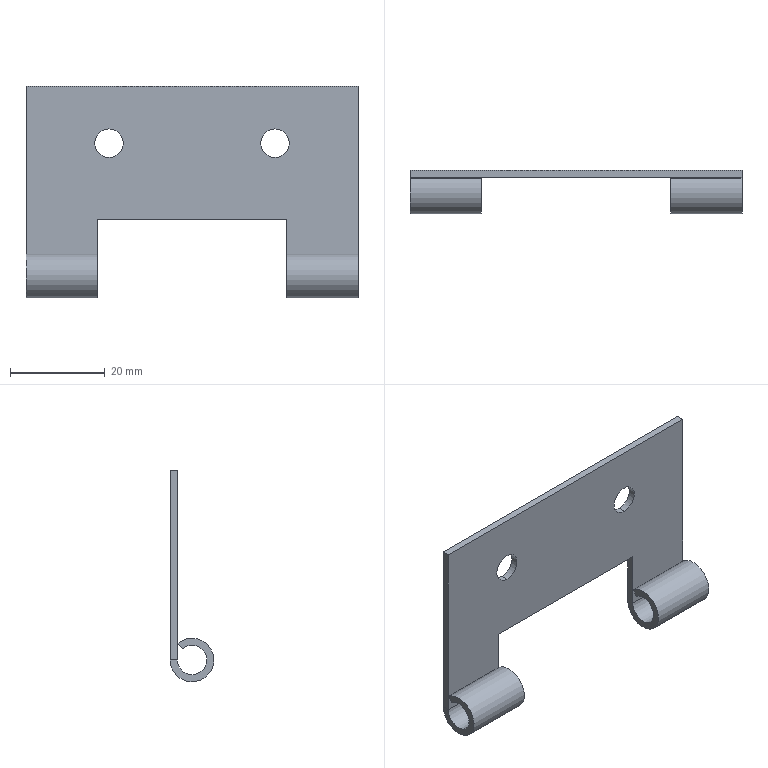Part | NX | features BREP 1 | 1 solid | 20 faces | box 70 x 9.2 x 44.6 mm | volume 4333 mm3 | plane 12 | cylinder 8 | commonest cylinder face diameters 6 x4 6.2 x2 9.2 x2
STEP:
#1=CARTESIAN_POINT('',(-20.,-1.5,-8.));
#2=VERTEX_POINT('',#1);
#3=CARTESIAN_POINT('',(-20.,-1.5,-20.));
#4=VERTEX_POINT('',#3);
#5=CARTESIAN_POINT('',(-20.,-1.5,-8.));
#6=DIRECTION('',(0.,0.,-1.));
#7=VECTOR('',#6,1000.);
#8=LINE('',#5,#7);
#9=EDGE_CURVE('',#2,#4,#8,.T.);
#10=ORIENTED_EDGE('',*,*,#9,.F.);
#11=CARTESIAN_POINT('',(20.,-1.5,-8.));
#12=VERTEX_POINT('',#11);
#13=CARTESIAN_POINT('',(20.,-1.5,-8.));
#14=DIRECTION('',(-1.,0.,0.));
#15=VECTOR('',#14,1000.);
#16=LINE('',#13,#15);
#17=EDGE_CURVE('',#12,#2,#16,.T.);
#18=ORIENTED_EDGE('',*,*,#17,.F.);
#19=CARTESIAN_POINT('',(20.,-1.5,-20.));
#20=VERTEX_POINT('',#19);
#21=CARTESIAN_POINT('',(20.,-1.5,-20.));
#22=DIRECTION('',(0.,0.,1.));
#23=VECTOR('',#22,1000.);
#24=LINE('',#21,#23);
#25=EDGE_CURVE('',#20,#12,#24,.T.);
#26=ORIENTED_EDGE('',*,*,#25,.F.);
#27=CARTESIAN_POINT('',(35.,-1.5,-20.));
#28=VERTEX_POINT('',#27);
#29=CARTESIAN_POINT('',(20.,-1.5,-20.));
#30=DIRECTION('',(1.,0.,0.));
#31=VECTOR('',#30,1000.);
#32=LINE('',#29,#31);
#33=EDGE_CURVE('',#20,#28,#32,.T.);
#34=ORIENTED_EDGE('',*,*,#33,.T.);
#35=CARTESIAN_POINT('',(35.,-1.5,20.));
#36=VERTEX_POINT('',#35);
#37=CARTESIAN_POINT('',(35.,-1.5,20.));
#38=DIRECTION('',(0.,0.,-1.));
#39=VECTOR('',#38,1000.);
#40=LINE('',#37,#39);
#41=EDGE_CURVE('',#36,#28,#40,.T.);
#42=ORIENTED_EDGE('',*,*,#41,.F.);
#43=CARTESIAN_POINT('',(-35.,-1.5,20.));
#44=VERTEX_POINT('',#43);
#45=CARTESIAN_POINT('',(-35.,-1.5,20.));
#46=DIRECTION('',(1.,0.,0.));
#47=VECTOR('',#46,1000.);
#48=LINE('',#45,#47);
#49=EDGE_CURVE('',#44,#36,#48,.T.);
#50=ORIENTED_EDGE('',*,*,#49,.F.);
#51=CARTESIAN_POINT('',(-35.,-1.5,-20.));
#52=VERTEX_POINT('',#51);
#53=CARTESIAN_POINT('',(-35.,-1.5,-20.));
#54=DIRECTION('',(0.,0.,1.));
#55=VECTOR('',#54,1000.);
#56=LINE('',#53,#55);
#57=EDGE_CURVE('',#52,#44,#56,.T.);
#58=ORIENTED_EDGE('',*,*,#57,.F.);
#59=CARTESIAN_POINT('',(-35.,-1.5,-20.));
#60=DIRECTION('',(1.,0.,0.));
#61=VECTOR('',#60,1000.);
#62=LINE('',#59,#61);
#63=EDGE_CURVE('',#52,#4,#62,.T.);
#64=ORIENTED_EDGE('',*,*,#63,.T.);
#65=EDGE_LOOP('',(#10,#18,#26,#34,#42,#50,#58,#64));
#66=FACE_BOUND('',#65,.T.);
#67=CARTESIAN_POINT('',(17.5,-1.5,5.));
#68=VERTEX_POINT('',#67);
#69=CARTESIAN_POINT('',(17.5,-1.5,11.));
#70=VERTEX_POINT('',#69);
#71=CARTESIAN_POINT('',(17.5,-1.5,8.));
#72=DIRECTION('',(0.,-1.,0.));
#73=DIRECTION('',(0.,0.,-1.));
#74=AXIS2_PLACEMENT_3D('',#71,#72,#73);
#75=CIRCLE('',#74,3.);
#76=EDGE_CURVE('',#68,#70,#75,.T.);
#77=ORIENTED_EDGE('',*,*,#76,.F.);
#78=CARTESIAN_POINT('',(17.5,-1.5,8.));
#79=DIRECTION('',(0.,-1.,0.));
#80=DIRECTION('',(0.,0.,1.));
#81=AXIS2_PLACEMENT_3D('',#78,#79,#80);
#82=CIRCLE('',#81,3.);
#83=EDGE_CURVE('',#70,#68,#82,.T.);
#84=ORIENTED_EDGE('',*,*,#83,.F.);
#85=EDGE_LOOP('',(#77,#84));
#86=FACE_BOUND('',#85,.T.);
#87=CARTESIAN_POINT('',(-17.5,-1.5,5.));
#88=VERTEX_POINT('',#87);
#89=CARTESIAN_POINT('',(-17.5,-1.5,11.));
#90=VERTEX_POINT('',#89);
#91=CARTESIAN_POINT('',(-17.5,-1.5,8.));
#92=DIRECTION('',(0.,-1.,0.));
#93=DIRECTION('',(0.,0.,-1.));
#94=AXIS2_PLACEMENT_3D('',#91,#92,#93);
#95=CIRCLE('',#94,3.);
#96=EDGE_CURVE('',#88,#90,#95,.T.);
#97=ORIENTED_EDGE('',*,*,#96,.F.);
#98=CARTESIAN_POINT('',(-17.5,-1.5,8.));
#99=DIRECTION('',(0.,-1.,0.));
#100=DIRECTION('',(0.,0.,1.));
#101=AXIS2_PLACEMENT_3D('',#98,#99,#100);
#102=CIRCLE('',#101,3.);
#103=EDGE_CURVE('',#90,#88,#102,.T.);
#104=ORIENTED_EDGE('',*,*,#103,.F.);
#105=EDGE_LOOP('',(#97,#104));
#106=FACE_BOUND('',#105,.T.);
#107=CARTESIAN_POINT('',(0.,-1.5,0.));
#108=DIRECTION('',(0.,-1.,0.));
#109=DIRECTION('',(0.,0.,-1.));
#110=AXIS2_PLACEMENT_3D('',#107,#108,#109);
#111=PLANE('',#110);
#112=ADVANCED_FACE('',(#66,#86,#106),#111,.T.);
#113=CARTESIAN_POINT('',(-20.,-2.607,-17.625));
#114=VERTEX_POINT('',#113);
#115=CARTESIAN_POINT('',(-20.,-4.6,-20.));
#116=DIRECTION('',(1.,0.,0.));
#117=DIRECTION('',(0.,0.,1.));
#118=AXIS2_PLACEMENT_3D('',#115,#116,#117);
#119=CIRCLE('',#118,3.1);
#120=EDGE_CURVE('',#114,#4,#119,.T.);
#121=ORIENTED_EDGE('',*,*,#120,.T.);
#122=ORIENTED_EDGE('',*,*,#63,.F.);
#123=CARTESIAN_POINT('',(-35.,-2.607,-17.625));
#124=VERTEX_POINT('',#123);
#125=CARTESIAN_POINT('',(-35.,-4.6,-20.));
#126=DIRECTION('',(-1.,0.,0.));
#127=DIRECTION('',(0.,1.,0.));
#128=AXIS2_PLACEMENT_3D('',#125,#126,#127);
#129=CIRCLE('',#128,3.1);
#130=EDGE_CURVE('',#52,#124,#129,.T.);
#131=ORIENTED_EDGE('',*,*,#130,.T.);
#132=CARTESIAN_POINT('',(-20.,-2.607,-17.625));
#133=DIRECTION('',(-1.,0.,0.));
#134=VECTOR('',#133,1000.);
#135=LINE('',#132,#134);
#136=EDGE_CURVE('',#114,#124,#135,.T.);
#137=ORIENTED_EDGE('',*,*,#136,.F.);
#138=EDGE_LOOP('',(#121,#122,#131,#137));
#139=FACE_BOUND('',#138,.T.);
#140=CARTESIAN_POINT('',(35.,-4.6,-20.));
#141=DIRECTION('',(1.,0.,0.));
#142=DIRECTION('',(0.,0.6428,0.766));
#143=AXIS2_PLACEMENT_3D('',#140,#141,#142);
#144=CYLINDRICAL_SURFACE('',#143,3.1);
#145=ADVANCED_FACE('',(#139),#144,.F.);
#146=CARTESIAN_POINT('',(-20.,0.,-8.));
#147=VERTEX_POINT('',#146);
#148=CARTESIAN_POINT('',(-20.,-1.5,-8.));
#149=DIRECTION('',(0.,1.,0.));
#150=VECTOR('',#149,1000.);
#151=LINE('',#148,#150);
#152=EDGE_CURVE('',#2,#147,#151,.T.);
#153=ORIENTED_EDGE('',*,*,#152,.F.);
#154=ORIENTED_EDGE('',*,*,#9,.T.);
#155=ORIENTED_EDGE('',*,*,#120,.F.);
#156=CARTESIAN_POINT('',(-20.,-1.643,-16.476));
#157=VERTEX_POINT('',#156);
#158=CARTESIAN_POINT('',(-20.,-1.643,-16.476));
#159=DIRECTION('',(0.,-0.6428,-0.766));
#160=VECTOR('',#159,1000.);
#161=LINE('',#158,#160);
#162=EDGE_CURVE('',#157,#114,#161,.T.);
#163=ORIENTED_EDGE('',*,*,#162,.F.);
#164=CARTESIAN_POINT('',(-20.,0.,-20.));
#165=VERTEX_POINT('',#164);
#166=CARTESIAN_POINT('',(-20.,-4.6,-20.));
#167=DIRECTION('',(-1.,0.,0.));
#168=DIRECTION('',(0.,0.,1.));
#169=AXIS2_PLACEMENT_3D('',#166,#167,#168);
#170=CIRCLE('',#169,4.6);
#171=EDGE_CURVE('',#165,#157,#170,.T.);
#172=ORIENTED_EDGE('',*,*,#171,.F.);
#173=CARTESIAN_POINT('',(-20.,0.,-20.));
#174=DIRECTION('',(0.,0.,1.));
#175=VECTOR('',#174,1000.);
#176=LINE('',#173,#175);
#177=EDGE_CURVE('',#165,#147,#176,.T.);
#178=ORIENTED_EDGE('',*,*,#177,.T.);
#179=EDGE_LOOP('',(#153,#154,#155,#163,#172,#178));
#180=FACE_BOUND('',#179,.T.);
#181=CARTESIAN_POINT('',(-20.,0.,-59.596));
#182=DIRECTION('',(1.,0.,0.));
#183=DIRECTION('',(0.,1.,0.));
#184=AXIS2_PLACEMENT_3D('',#181,#182,#183);
#185=PLANE('',#184);
#186=ADVANCED_FACE('',(#180),#185,.T.);
#187=CARTESIAN_POINT('',(-35.,0.,-20.));
#188=VERTEX_POINT('',#187);
#189=CARTESIAN_POINT('',(-20.,0.,-20.));
#190=DIRECTION('',(-1.,0.,0.));
#191=VECTOR('',#190,1000.);
#192=LINE('',#189,#191);
#193=EDGE_CURVE('',#165,#188,#192,.T.);
#194=ORIENTED_EDGE('',*,*,#193,.T.);
#195=CARTESIAN_POINT('',(-35.,0.,20.));
#196=VERTEX_POINT('',#195);
#197=CARTESIAN_POINT('',(-35.,0.,20.));
#198=DIRECTION('',(0.,0.,-1.));
#199=VECTOR('',#198,1000.);
#200=LINE('',#197,#199);
#201=EDGE_CURVE('',#196,#188,#200,.T.);
#202=ORIENTED_EDGE('',*,*,#201,.F.);
#203=CARTESIAN_POINT('',(35.,0.,20.));
#204=VERTEX_POINT('',#203);
#205=CARTESIAN_POINT('',(35.,0.,20.));
#206=DIRECTION('',(-1.,0.,0.));
#207=VECTOR('',#206,1000.);
#208=LINE('',#205,#207);
#209=EDGE_CURVE('',#204,#196,#208,.T.);
#210=ORIENTED_EDGE('',*,*,#209,.F.);
#211=CARTESIAN_POINT('',(35.,0.,-20.));
#212=VERTEX_POINT('',#211);
#213=CARTESIAN_POINT('',(35.,0.,-20.));
#214=DIRECTION('',(0.,0.,1.));
#215=VECTOR('',#214,1000.);
#216=LINE('',#213,#215);
#217=EDGE_CURVE('',#212,#204,#216,.T.);
#218=ORIENTED_EDGE('',*,*,#217,.F.);
#219=CARTESIAN_POINT('',(20.,0.,-20.));
#220=VERTEX_POINT('',#219);
#221=CARTESIAN_POINT('',(35.,0.,-20.));
#222=DIRECTION('',(-1.,0.,0.));
#223=VECTOR('',#222,1000.);
#224=LINE('',#221,#223);
#225=EDGE_CURVE('',#212,#220,#224,.T.);
#226=ORIENTED_EDGE('',*,*,#225,.T.);
#227=CARTESIAN_POINT('',(20.,0.,-8.));
#228=VERTEX_POINT('',#227);
#229=CARTESIAN_POINT('',(20.,0.,-8.));
#230=DIRECTION('',(0.,0.,-1.));
#231=VECTOR('',#230,1000.);
#232=LINE('',#229,#231);
#233=EDGE_CURVE('',#228,#220,#232,.T.);
#234=ORIENTED_EDGE('',*,*,#233,.F.);
#235=CARTESIAN_POINT('',(-20.,0.,-8.));
#236=DIRECTION('',(1.,0.,0.));
#237=VECTOR('',#236,1000.);
#238=LINE('',#235,#237);
#239=EDGE_CURVE('',#147,#228,#238,.T.);
#240=ORIENTED_EDGE('',*,*,#239,.F.);
#241=ORIENTED_EDGE('',*,*,#177,.F.);
#242=EDGE_LOOP('',(#194,#202,#210,#218,#226,#234,#240,#241));
#243=FACE_BOUND('',#242,.T.);
#244=CARTESIAN_POINT('',(17.5,0.,5.));
#245=VERTEX_POINT('',#244);
#246=CARTESIAN_POINT('',(17.5,0.,11.));
#247=VERTEX_POINT('',#246);
#248=CARTESIAN_POINT('',(17.5,0.,8.));
#249=DIRECTION('',(0.,1.,0.));
#250=DIRECTION('',(0.,0.,-1.));
#251=AXIS2_PLACEMENT_3D('',#248,#249,#250);
#252=CIRCLE('',#251,3.);
#253=EDGE_CURVE('',#245,#247,#252,.T.);
#254=ORIENTED_EDGE('',*,*,#253,.F.);
#255=CARTESIAN_POINT('',(17.5,0.,8.));
#256=DIRECTION('',(0.,1.,0.));
#257=DIRECTION('',(0.,0.,1.));
#258=AXIS2_PLACEMENT_3D('',#255,#256,#257);
#259=CIRCLE('',#258,3.);
#260=EDGE_CURVE('',#247,#245,#259,.T.);
#261=ORIENTED_EDGE('',*,*,#260,.F.);
#262=EDGE_LOOP('',(#254,#261));
#263=FACE_BOUND('',#262,.T.);
#264=CARTESIAN_POINT('',(-17.5,0.,5.));
#265=VERTEX_POINT('',#264);
#266=CARTESIAN_POINT('',(-17.5,0.,11.));
#267=VERTEX_POINT('',#266);
#268=CARTESIAN_POINT('',(-17.5,0.,8.));
#269=DIRECTION('',(0.,1.,0.));
#270=DIRECTION('',(0.,0.,-1.));
#271=AXIS2_PLACEMENT_3D('',#268,#269,#270);
#272=CIRCLE('',#271,3.);
#273=EDGE_CURVE('',#265,#267,#272,.T.);
#274=ORIENTED_EDGE('',*,*,#273,.F.);
#275=CARTESIAN_POINT('',(-17.5,0.,8.));
#276=DIRECTION('',(0.,1.,0.));
#277=DIRECTION('',(0.,0.,1.));
#278=AXIS2_PLACEMENT_3D('',#275,#276,#277);
#279=CIRCLE('',#278,3.);
#280=EDGE_CURVE('',#267,#265,#279,.T.);
#281=ORIENTED_EDGE('',*,*,#280,.F.);
#282=EDGE_LOOP('',(#274,#281));
#283=FACE_BOUND('',#282,.T.);
#284=CARTESIAN_POINT('',(0.,0.,0.));
#285=DIRECTION('',(0.,-1.,0.));
#286=DIRECTION('',(0.,0.,-1.));
#287=AXIS2_PLACEMENT_3D('',#284,#285,#286);
#288=PLANE('',#287);
#289=ADVANCED_FACE('',(#243,#263,#283),#288,.F.);
#290=ORIENTED_EDGE('',*,*,#239,.T.);
#291=CARTESIAN_POINT('',(20.,-1.5,-8.));
#292=DIRECTION('',(0.,1.,0.));
#293=VECTOR('',#292,1000.);
#294=LINE('',#291,#293);
#295=EDGE_CURVE('',#12,#228,#294,.T.);
#296=ORIENTED_EDGE('',*,*,#295,.F.);
#297=ORIENTED_EDGE('',*,*,#17,.T.);
#298=ORIENTED_EDGE('',*,*,#152,.T.);
#299=EDGE_LOOP('',(#290,#296,#297,#298));
#300=FACE_BOUND('',#299,.T.);
#301=CARTESIAN_POINT('',(-20.,0.,-8.));
#302=DIRECTION('',(0.,0.,-1.));
#303=DIRECTION('',(0.,-1.,0.));
#304=AXIS2_PLACEMENT_3D('',#301,#302,#303);
#305=PLANE('',#304);
#306=ADVANCED_FACE('',(#300),#305,.T.);
#307=CARTESIAN_POINT('',(20.,-1.643,-16.476));
#308=VERTEX_POINT('',#307);
#309=CARTESIAN_POINT('',(20.,-4.6,-20.));
#310=DIRECTION('',(1.,0.,0.));
#311=DIRECTION('',(0.,0.,1.));
#312=AXIS2_PLACEMENT_3D('',#309,#310,#311);
#313=CIRCLE('',#312,4.6);
#314=EDGE_CURVE('',#308,#220,#313,.T.);
#315=ORIENTED_EDGE('',*,*,#314,.F.);
#316=CARTESIAN_POINT('',(20.,-2.607,-17.625));
#317=VERTEX_POINT('',#316);
#318=CARTESIAN_POINT('',(20.,-2.607,-17.625));
#319=DIRECTION('',(0.,0.6428,0.766));
#320=VECTOR('',#319,1000.);
#321=LINE('',#318,#320);
#322=EDGE_CURVE('',#317,#308,#321,.T.);
#323=ORIENTED_EDGE('',*,*,#322,.F.);
#324=CARTESIAN_POINT('',(20.,-4.6,-20.));
#325=DIRECTION('',(-1.,0.,0.));
#326=DIRECTION('',(0.,0.,1.));
#327=AXIS2_PLACEMENT_3D('',#324,#325,#326);
#328=CIRCLE('',#327,3.1);
#329=EDGE_CURVE('',#20,#317,#328,.T.);
#330=ORIENTED_EDGE('',*,*,#329,.F.);
#331=ORIENTED_EDGE('',*,*,#25,.T.);
#332=ORIENTED_EDGE('',*,*,#295,.T.);
#333=ORIENTED_EDGE('',*,*,#233,.T.);
#334=EDGE_LOOP('',(#315,#323,#330,#331,#332,#333));
#335=FACE_BOUND('',#334,.T.);
#336=CARTESIAN_POINT('',(20.,0.,-59.596));
#337=DIRECTION('',(1.,0.,0.));
#338=DIRECTION('',(0.,1.,0.));
#339=AXIS2_PLACEMENT_3D('',#336,#337,#338);
#340=PLANE('',#339);
#341=ADVANCED_FACE('',(#335),#340,.F.);
#342=CARTESIAN_POINT('',(35.,-1.643,-16.476));
#343=VERTEX_POINT('',#342);
#344=CARTESIAN_POINT('',(20.,-1.643,-16.476));
#345=DIRECTION('',(1.,0.,0.));
#346=VECTOR('',#345,1000.);
#347=LINE('',#344,#346);
#348=EDGE_CURVE('',#308,#343,#347,.T.);
#349=ORIENTED_EDGE('',*,*,#348,.F.);
#350=ORIENTED_EDGE('',*,*,#314,.T.);
#351=ORIENTED_EDGE('',*,*,#225,.F.);
#352=CARTESIAN_POINT('',(35.,-4.6,-20.));
#353=DIRECTION('',(-1.,0.,0.));
#354=DIRECTION('',(0.,1.,0.));
#355=AXIS2_PLACEMENT_3D('',#352,#353,#354);
#356=CIRCLE('',#355,4.6);
#357=EDGE_CURVE('',#212,#343,#356,.T.);
#358=ORIENTED_EDGE('',*,*,#357,.T.);
#359=EDGE_LOOP('',(#349,#350,#351,#358));
#360=FACE_BOUND('',#359,.T.);
#361=CARTESIAN_POINT('',(35.,-4.6,-20.));
#362=DIRECTION('',(1.,0.,0.));
#363=DIRECTION('',(0.,0.6428,0.766));
#364=AXIS2_PLACEMENT_3D('',#361,#362,#363);
#365=CYLINDRICAL_SURFACE('',#364,4.6);
#366=ADVANCED_FACE('',(#360),#365,.T.);
#367=ORIENTED_EDGE('',*,*,#348,.T.);
#368=CARTESIAN_POINT('',(35.,-2.607,-17.625));
#369=VERTEX_POINT('',#368);
#370=CARTESIAN_POINT('',(35.,-1.643,-16.476));
#371=DIRECTION('',(0.,-0.6428,-0.766));
#372=VECTOR('',#371,1000.);
#373=LINE('',#370,#372);
#374=EDGE_CURVE('',#343,#369,#373,.T.);
#375=ORIENTED_EDGE('',*,*,#374,.T.);
#376=CARTESIAN_POINT('',(35.,-2.607,-17.625));
#377=DIRECTION('',(-1.,0.,0.));
#378=VECTOR('',#377,1000.);
#379=LINE('',#376,#378);
#380=EDGE_CURVE('',#369,#317,#379,.T.);
#381=ORIENTED_EDGE('',*,*,#380,.T.);
#382=ORIENTED_EDGE('',*,*,#322,.T.);
#383=EDGE_LOOP('',(#367,#375,#381,#382));
#384=FACE_BOUND('',#383,.T.);
#385=CARTESIAN_POINT('',(0.,-2.607,-17.625));
#386=DIRECTION('',(0.,-0.766,0.6428));
#387=DIRECTION('',(-1.,0.,0.));
#388=AXIS2_PLACEMENT_3D('',#385,#386,#387);
#389=PLANE('',#388);
#390=ADVANCED_FACE('',(#384),#389,.F.);
#391=ORIENTED_EDGE('',*,*,#33,.F.);
#392=ORIENTED_EDGE('',*,*,#329,.T.);
#393=ORIENTED_EDGE('',*,*,#380,.F.);
#394=CARTESIAN_POINT('',(35.,-4.6,-20.));
#395=DIRECTION('',(1.,0.,0.));
#396=DIRECTION('',(0.,0.6428,0.766));
#397=AXIS2_PLACEMENT_3D('',#394,#395,#396);
#398=CIRCLE('',#397,3.1);
#399=EDGE_CURVE('',#369,#28,#398,.T.);
#400=ORIENTED_EDGE('',*,*,#399,.T.);
#401=EDGE_LOOP('',(#391,#392,#393,#400));
#402=FACE_BOUND('',#401,.T.);
#403=CARTESIAN_POINT('',(35.,-4.6,-20.));
#404=DIRECTION('',(1.,0.,0.));
#405=DIRECTION('',(0.,0.6428,0.766));
#406=AXIS2_PLACEMENT_3D('',#403,#404,#405);
#407=CYLINDRICAL_SURFACE('',#406,3.1);
#408=ADVANCED_FACE('',(#402),#407,.F.);
#409=ORIENTED_EDGE('',*,*,#399,.F.);
#410=ORIENTED_EDGE('',*,*,#374,.F.);
#411=ORIENTED_EDGE('',*,*,#357,.F.);
#412=CARTESIAN_POINT('',(35.,0.,-20.));
#413=DIRECTION('',(0.,-1.,0.));
#414=VECTOR('',#413,1000.);
#415=LINE('',#412,#414);
#416=EDGE_CURVE('',#212,#28,#415,.T.);
#417=ORIENTED_EDGE('',*,*,#416,.T.);
#418=EDGE_LOOP('',(#409,#410,#411,#417));
#419=FACE_BOUND('',#418,.T.);
#420=CARTESIAN_POINT('',(35.,-4.6,-20.));
#421=DIRECTION('',(-1.,0.,0.));
#422=DIRECTION('',(0.,0.,1.));
#423=AXIS2_PLACEMENT_3D('',#420,#421,#422);
#424=PLANE('',#423);
#425=ADVANCED_FACE('',(#419),#424,.F.);
#426=CARTESIAN_POINT('',(35.,-1.5,20.));
#427=DIRECTION('',(0.,1.,0.));
#428=VECTOR('',#427,1000.);
#429=LINE('',#426,#428);
#430=EDGE_CURVE('',#36,#204,#429,.T.);
#431=ORIENTED_EDGE('',*,*,#430,.F.);
#432=ORIENTED_EDGE('',*,*,#41,.T.);
#433=ORIENTED_EDGE('',*,*,#416,.F.);
#434=ORIENTED_EDGE('',*,*,#217,.T.);
#435=EDGE_LOOP('',(#431,#432,#433,#434));
#436=FACE_BOUND('',#435,.T.);
#437=CARTESIAN_POINT('',(35.,-1.5,20.));
#438=DIRECTION('',(1.,0.,0.));
#439=DIRECTION('',(0.,1.,0.));
#440=AXIS2_PLACEMENT_3D('',#437,#438,#439);
#441=PLANE('',#440);
#442=ADVANCED_FACE('',(#436),#441,.T.);
#443=CARTESIAN_POINT('',(-35.,-1.5,20.));
#444=DIRECTION('',(0.,1.,0.));
#445=VECTOR('',#444,1000.);
#446=LINE('',#443,#445);
#447=EDGE_CURVE('',#44,#196,#446,.T.);
#448=ORIENTED_EDGE('',*,*,#447,.F.);
#449=ORIENTED_EDGE('',*,*,#49,.T.);
#450=ORIENTED_EDGE('',*,*,#430,.T.);
#451=ORIENTED_EDGE('',*,*,#209,.T.);
#452=EDGE_LOOP('',(#448,#449,#450,#451));
#453=FACE_BOUND('',#452,.T.);
#454=CARTESIAN_POINT('',(-35.,-1.5,20.));
#455=DIRECTION('',(0.,0.,1.));
#456=DIRECTION('',(1.,0.,0.));
#457=AXIS2_PLACEMENT_3D('',#454,#455,#456);
#458=PLANE('',#457);
#459=ADVANCED_FACE('',(#453),#458,.T.);
#460=CARTESIAN_POINT('',(-35.,-1.5,-20.));
#461=DIRECTION('',(0.,1.,0.));
#462=VECTOR('',#461,1000.);
#463=LINE('',#460,#462);
#464=EDGE_CURVE('',#52,#188,#463,.T.);
#465=ORIENTED_EDGE('',*,*,#464,.F.);
#466=ORIENTED_EDGE('',*,*,#57,.T.);
#467=ORIENTED_EDGE('',*,*,#447,.T.);
#468=ORIENTED_EDGE('',*,*,#201,.T.);
#469=EDGE_LOOP('',(#465,#466,#467,#468));
#470=FACE_BOUND('',#469,.T.);
#471=CARTESIAN_POINT('',(-35.,-1.5,20.));
#472=DIRECTION('',(-1.,0.,0.));
#473=DIRECTION('',(0.,0.,1.));
#474=AXIS2_PLACEMENT_3D('',#471,#472,#473);
#475=PLANE('',#474);
#476=ADVANCED_FACE('',(#470),#475,.T.);
#477=CARTESIAN_POINT('',(-35.,-1.643,-16.476));
#478=VERTEX_POINT('',#477);
#479=CARTESIAN_POINT('',(-35.,-2.607,-17.625));
#480=DIRECTION('',(0.,0.6428,0.766));
#481=VECTOR('',#480,1000.);
#482=LINE('',#479,#481);
#483=EDGE_CURVE('',#124,#478,#482,.T.);
#484=ORIENTED_EDGE('',*,*,#483,.F.);
#485=ORIENTED_EDGE('',*,*,#130,.F.);
#486=ORIENTED_EDGE('',*,*,#464,.T.);
#487=CARTESIAN_POINT('',(-35.,-4.6,-20.));
#488=DIRECTION('',(1.,0.,0.));
#489=DIRECTION('',(0.,-0.6428,-0.766));
#490=AXIS2_PLACEMENT_3D('',#487,#488,#489);
#491=CIRCLE('',#490,4.6);
#492=EDGE_CURVE('',#478,#188,#491,.T.);
#493=ORIENTED_EDGE('',*,*,#492,.F.);
#494=EDGE_LOOP('',(#484,#485,#486,#493));
#495=FACE_BOUND('',#494,.T.);
#496=CARTESIAN_POINT('',(-35.,-4.6,-20.));
#497=DIRECTION('',(-1.,0.,0.));
#498=DIRECTION('',(0.,0.,1.));
#499=AXIS2_PLACEMENT_3D('',#496,#497,#498);
#500=PLANE('',#499);
#501=ADVANCED_FACE('',(#495),#500,.T.);
#502=ORIENTED_EDGE('',*,*,#162,.T.);
#503=ORIENTED_EDGE('',*,*,#136,.T.);
#504=ORIENTED_EDGE('',*,*,#483,.T.);
#505=CARTESIAN_POINT('',(-35.,-1.643,-16.476));
#506=DIRECTION('',(1.,0.,0.));
#507=VECTOR('',#506,1000.);
#508=LINE('',#505,#507);
#509=EDGE_CURVE('',#478,#157,#508,.T.);
#510=ORIENTED_EDGE('',*,*,#509,.T.);
#511=EDGE_LOOP('',(#502,#503,#504,#510));
#512=FACE_BOUND('',#511,.T.);
#513=CARTESIAN_POINT('',(0.,-2.607,-17.625));
#514=DIRECTION('',(0.,-0.766,0.6428));
#515=DIRECTION('',(-1.,0.,0.));
#516=AXIS2_PLACEMENT_3D('',#513,#514,#515);
#517=PLANE('',#516);
#518=ADVANCED_FACE('',(#512),#517,.F.);
#519=ORIENTED_EDGE('',*,*,#193,.F.);
#520=ORIENTED_EDGE('',*,*,#171,.T.);
#521=ORIENTED_EDGE('',*,*,#509,.F.);
#522=ORIENTED_EDGE('',*,*,#492,.T.);
#523=EDGE_LOOP('',(#519,#520,#521,#522));
#524=FACE_BOUND('',#523,.T.);
#525=CARTESIAN_POINT('',(35.,-4.6,-20.));
#526=DIRECTION('',(1.,0.,0.));
#527=DIRECTION('',(0.,0.6428,0.766));
#528=AXIS2_PLACEMENT_3D('',#525,#526,#527);
#529=CYLINDRICAL_SURFACE('',#528,4.6);
#530=ADVANCED_FACE('',(#524),#529,.T.);
#531=CARTESIAN_POINT('',(17.5,-1.5,11.));
#532=DIRECTION('',(0.,1.,0.));
#533=VECTOR('',#532,1000.);
#534=LINE('',#531,#533);
#535=EDGE_CURVE('',#247,#70,#534,.F.);
#536=ORIENTED_EDGE('',*,*,#535,.F.);
#537=ORIENTED_EDGE('',*,*,#260,.T.);
#538=CARTESIAN_POINT('',(17.5,-1.5,5.));
#539=DIRECTION('',(0.,1.,0.));
#540=VECTOR('',#539,1000.);
#541=LINE('',#538,#540);
#542=EDGE_CURVE('',#245,#68,#541,.F.);
#543=ORIENTED_EDGE('',*,*,#542,.T.);
#544=ORIENTED_EDGE('',*,*,#76,.T.);
#545=EDGE_LOOP('',(#536,#537,#543,#544));
#546=FACE_BOUND('',#545,.T.);
#547=CARTESIAN_POINT('',(17.5,8.5,8.));
#548=DIRECTION('',(0.,-1.,0.));
#549=DIRECTION('',(0.,0.,-1.));
#550=AXIS2_PLACEMENT_3D('',#547,#548,#549);
#551=CYLINDRICAL_SURFACE('',#550,3.);
#552=ADVANCED_FACE('',(#546),#551,.F.);
#553=ORIENTED_EDGE('',*,*,#542,.F.);
#554=ORIENTED_EDGE('',*,*,#253,.T.);
#555=ORIENTED_EDGE('',*,*,#535,.T.);
#556=ORIENTED_EDGE('',*,*,#83,.T.);
#557=EDGE_LOOP('',(#553,#554,#555,#556));
#558=FACE_BOUND('',#557,.T.);
#559=CARTESIAN_POINT('',(17.5,8.5,8.));
#560=DIRECTION('',(0.,-1.,0.));
#561=DIRECTION('',(0.,0.,-1.));
#562=AXIS2_PLACEMENT_3D('',#559,#560,#561);
#563=CYLINDRICAL_SURFACE('',#562,3.);
#564=ADVANCED_FACE('',(#558),#563,.F.);
#565=CARTESIAN_POINT('',(-17.5,-1.5,11.));
#566=DIRECTION('',(0.,1.,0.));
#567=VECTOR('',#566,1000.);
#568=LINE('',#565,#567);
#569=EDGE_CURVE('',#267,#90,#568,.F.);
#570=ORIENTED_EDGE('',*,*,#569,.F.);
#571=ORIENTED_EDGE('',*,*,#280,.T.);
#572=CARTESIAN_POINT('',(-17.5,-1.5,5.));
#573=DIRECTION('',(0.,1.,0.));
#574=VECTOR('',#573,1000.);
#575=LINE('',#572,#574);
#576=EDGE_CURVE('',#265,#88,#575,.F.);
#577=ORIENTED_EDGE('',*,*,#576,.T.);
#578=ORIENTED_EDGE('',*,*,#96,.T.);
#579=EDGE_LOOP('',(#570,#571,#577,#578));
#580=FACE_BOUND('',#579,.T.);
#581=CARTESIAN_POINT('',(-17.5,8.5,8.));
#582=DIRECTION('',(0.,-1.,0.));
#583=DIRECTION('',(0.,0.,-1.));
#584=AXIS2_PLACEMENT_3D('',#581,#582,#583);
#585=CYLINDRICAL_SURFACE('',#584,3.);
#586=ADVANCED_FACE('',(#580),#585,.F.);
#587=ORIENTED_EDGE('',*,*,#576,.F.);
#588=ORIENTED_EDGE('',*,*,#273,.T.);
#589=ORIENTED_EDGE('',*,*,#569,.T.);
#590=ORIENTED_EDGE('',*,*,#103,.T.);
#591=EDGE_LOOP('',(#587,#588,#589,#590));
#592=FACE_BOUND('',#591,.T.);
#593=CARTESIAN_POINT('',(-17.5,8.5,8.));
#594=DIRECTION('',(0.,-1.,0.));
#595=DIRECTION('',(0.,0.,-1.));
#596=AXIS2_PLACEMENT_3D('',#593,#594,#595);
#597=CYLINDRICAL_SURFACE('',#596,3.);
#598=ADVANCED_FACE('',(#592),#597,.F.);
#599=CLOSED_SHELL('',(#112,#145,#186,#289,#306,#341,#366,#390,#408,#425,#442,#459,#476,#501,#518,#530,#552,#564,#586,#598));
#600=MANIFOLD_SOLID_BREP('',#599);
#601=(LENGTH_UNIT()NAMED_UNIT(*)SI_UNIT(.MILLI.,.METRE.));
#602=UNCERTAINTY_MEASURE_WITH_UNIT(LENGTH_MEASURE(0.00001),#601,'','');
#603=(NAMED_UNIT(*)PLANE_ANGLE_UNIT()SI_UNIT($,.RADIAN.));
#604=(NAMED_UNIT(*)SI_UNIT($,.STERADIAN.)SOLID_ANGLE_UNIT());
#605=(GEOMETRIC_REPRESENTATION_CONTEXT(3)GLOBAL_UNCERTAINTY_ASSIGNED_CONTEXT((#602))GLOBAL_UNIT_ASSIGNED_CONTEXT((#601,#603,#604))REPRESENTATION_CONTEXT('',''));
#606=ADVANCED_BREP_SHAPE_REPRESENTATION('',(#600),#605);